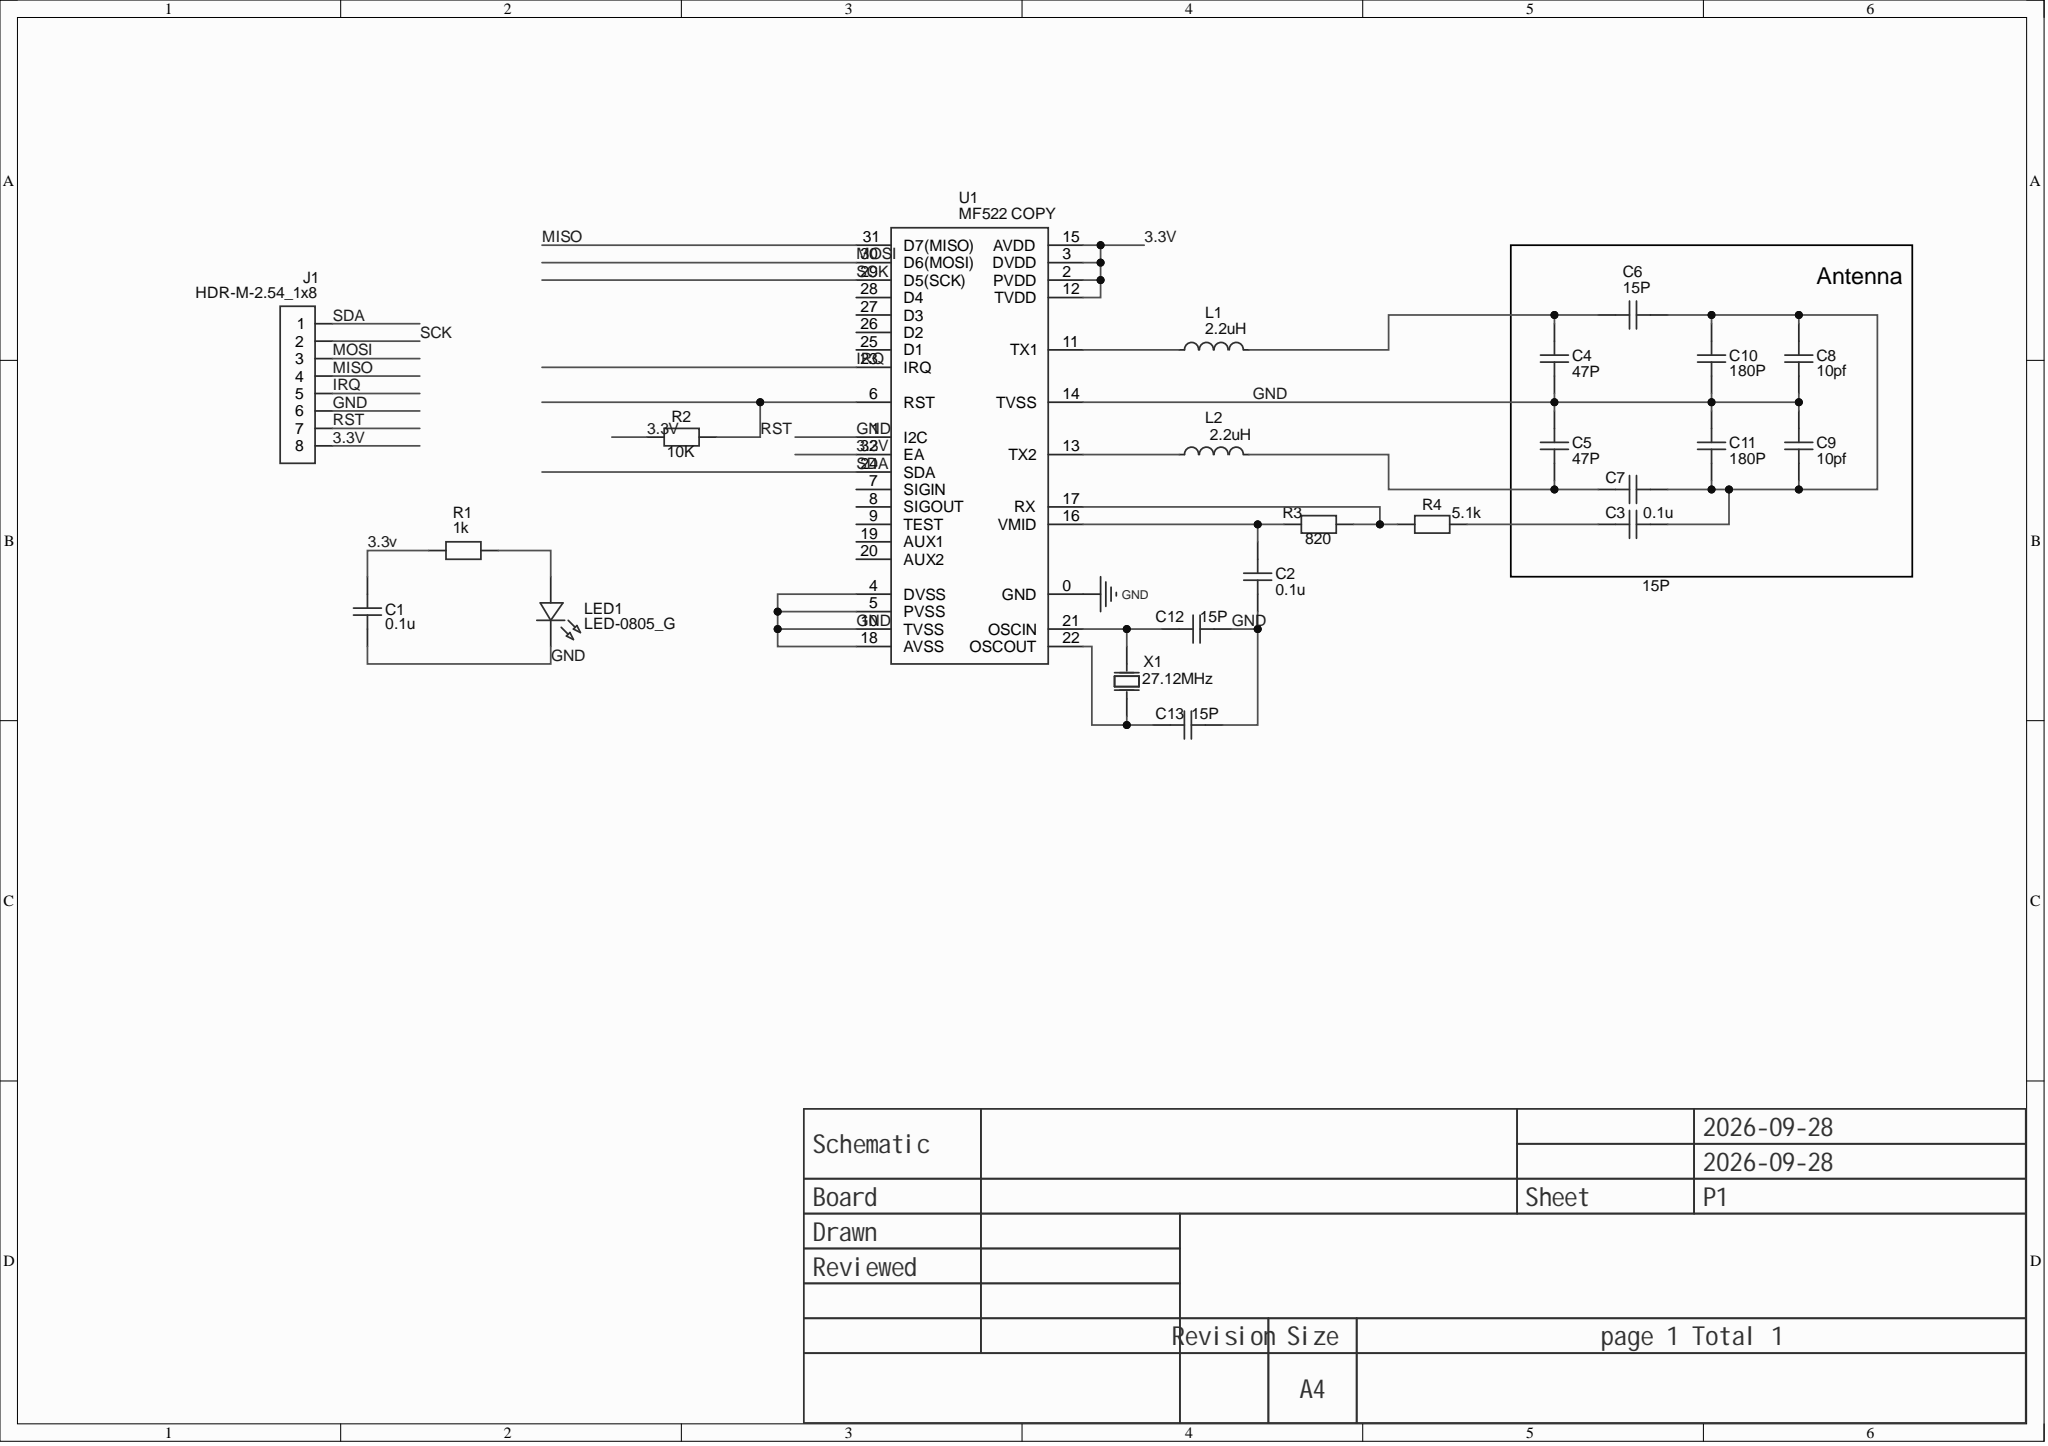Circuit board | Altium Designer | 23 parts | 19 nets
Bill of materials:
Comment,Description,Designator,Footprint,LibRef,Quantity
"0.1u","","C1, C2, C3","C0805","0.1u","3"
"47P","","C4, C5","C0805","47P","2"
"15P","","C6, C7, C12, C13","C0805","15P","4"
"10pf","","C8, C9","C0805","10pf","2"
"180P","","C10, C11","C0805","180P","2"
"HDR-M-2.54_1x8","","J1","HDR-M-2.54_1X8","HDR-M-2.54_1x8","1"
"2.2uH","","L1, L2","L0805","2.2uH","2"
"LED-0805_G","","LED1","LED-0805_G","NCD0805G1","1"
"1k","","R1","R0805","1k","1"
"10K","","R2","R0805","10K","1"
"820","","R3","R0805","820","1"
"5.1k","","R4","R0805","5.1k","1"
"MF522 COPY","","U1","LC-QFN-32_5X5X05P","MF522 COPY","1"
"27.12MHz","","X1","HC-49US_L11.5-W4.5-P4.88","X49UD196608MSD2SC","1"
Netlist (Protel format):
[
C1
C0805
0.1u



]
[
C2
C0805
0.1u



]
[
C3
C0805
0.1u



]
[
C4
C0805
47P



]
[
C5
C0805
47P



]
[
C6
C0805
15P



]
[
C7
C0805
15P



]
[
C8
C0805
10pf



]
[
C9
C0805
10pf



]
[
C10
C0805
180P



]
[
C11
C0805
180P



]
[
C12
C0805
15P



]
[
C13
C0805
15P



]
[
J1
HDR-M-2.54_1X8
HDR-M-2.54_1x8



]
[
L1
L0805
2.2uH



]
[
L2
L0805
2.2uH



]
[
LED1
LED-0805_G
LED-0805_G



]
[
R1
R0805
1k



]
[
R2
R0805
10K



]
[
R3
R0805
820



]
[
R4
R0805
5.1k



]
[
U1
LC-QFN-32_5X5X05P
MF522 COPY



]
[
X1
HC-49US_L11.5-W4.5-P4.88
27.12MHz



]
(
SDA
J1-1
U1-24
)
(
SCK
J1-2
U1-29
)
(
RST
J1-7
R2-2
U1-6
)
(
NetR3_2
R3-2
R4-1
U1-17
)
(
NetLED1_1
LED1-1
R1-2
)
(
NetL2_1
L2-1
U1-13
)
(
NetL1_1
L1-1
U1-11
)
(
NetC13_1
C13-1
U1-22
X1-2
)
(
NetC12_1
C12-1
U1-21
X1-1
)
(
NetC5_1
C5-1
C7-1
L2-2
)
(
NetC4_2
C4-2
C6-1
L1-2
)
(
NetC3_2
C3-2
C6-2
C7-2
C8-2
C9-1
C10-2
C11-1
)
(
NetC3_1
C3-1
R4-2
)
(
NetC2_2
C2-2
R3-1
U1-16
)
(
MOSI
J1-3
U1-30
)
(
MISO
J1-4
U1-31
)
(
IRQ
J1-5
U1-23
)
(
GND
C1-1
C2-1
C4-1
C5-2
C8-1
C9-2
C10-1
C11-2
C12-2
C13-2
J1-6
LED1-2
U1-0
U1-1
U1-4
U1-5
U1-10
U1-14
U1-18
)
(
3.3v
C1-2
J1-8
R1-1
R2-1
U1-2
U1-3
U1-12
U1-15
U1-32
)